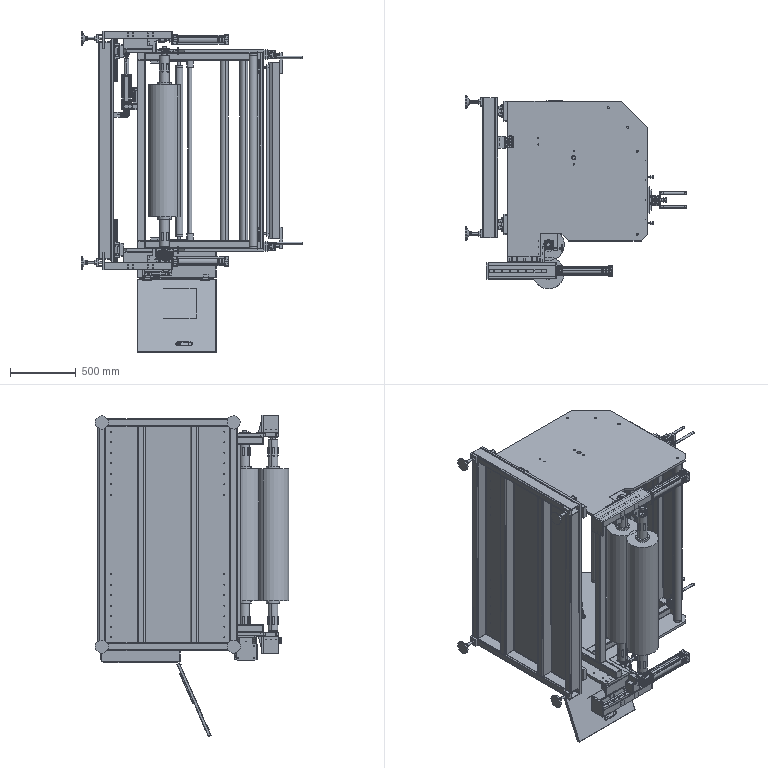Part | SolidWorks | features CompositeCurve 4 | 363 solids | 16137 faces | volume 235835811 mm3 | cylinder 5938 | plane 5877 | spline 1760 | cone 1368 | torus 786 | sphere 408 | commonest cylinder face diameters 0.4 x276 6.8 x270 41.25 x264 43.75 x264 9 x226 15 x210